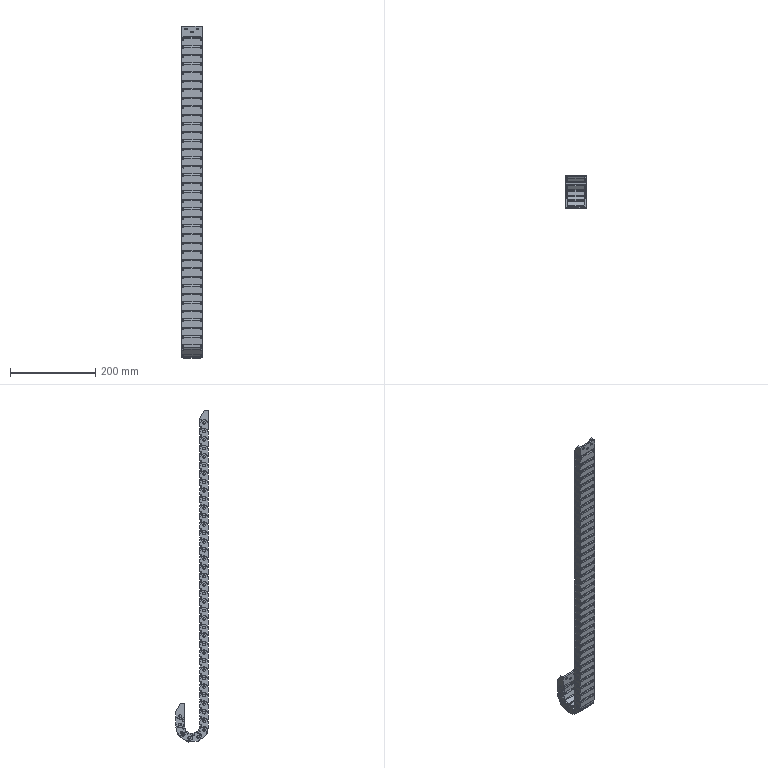Part | SolidWorks | features BaseBody 43 | 43 solids | 4034 faces | volume 252756 mm3 | plane 2563 | cylinder 1459 | cone 12 | commonest cylinder face diameters 0.4 x328 6 x168 6.3 x164 14 x160 15.2 x154 4 x117